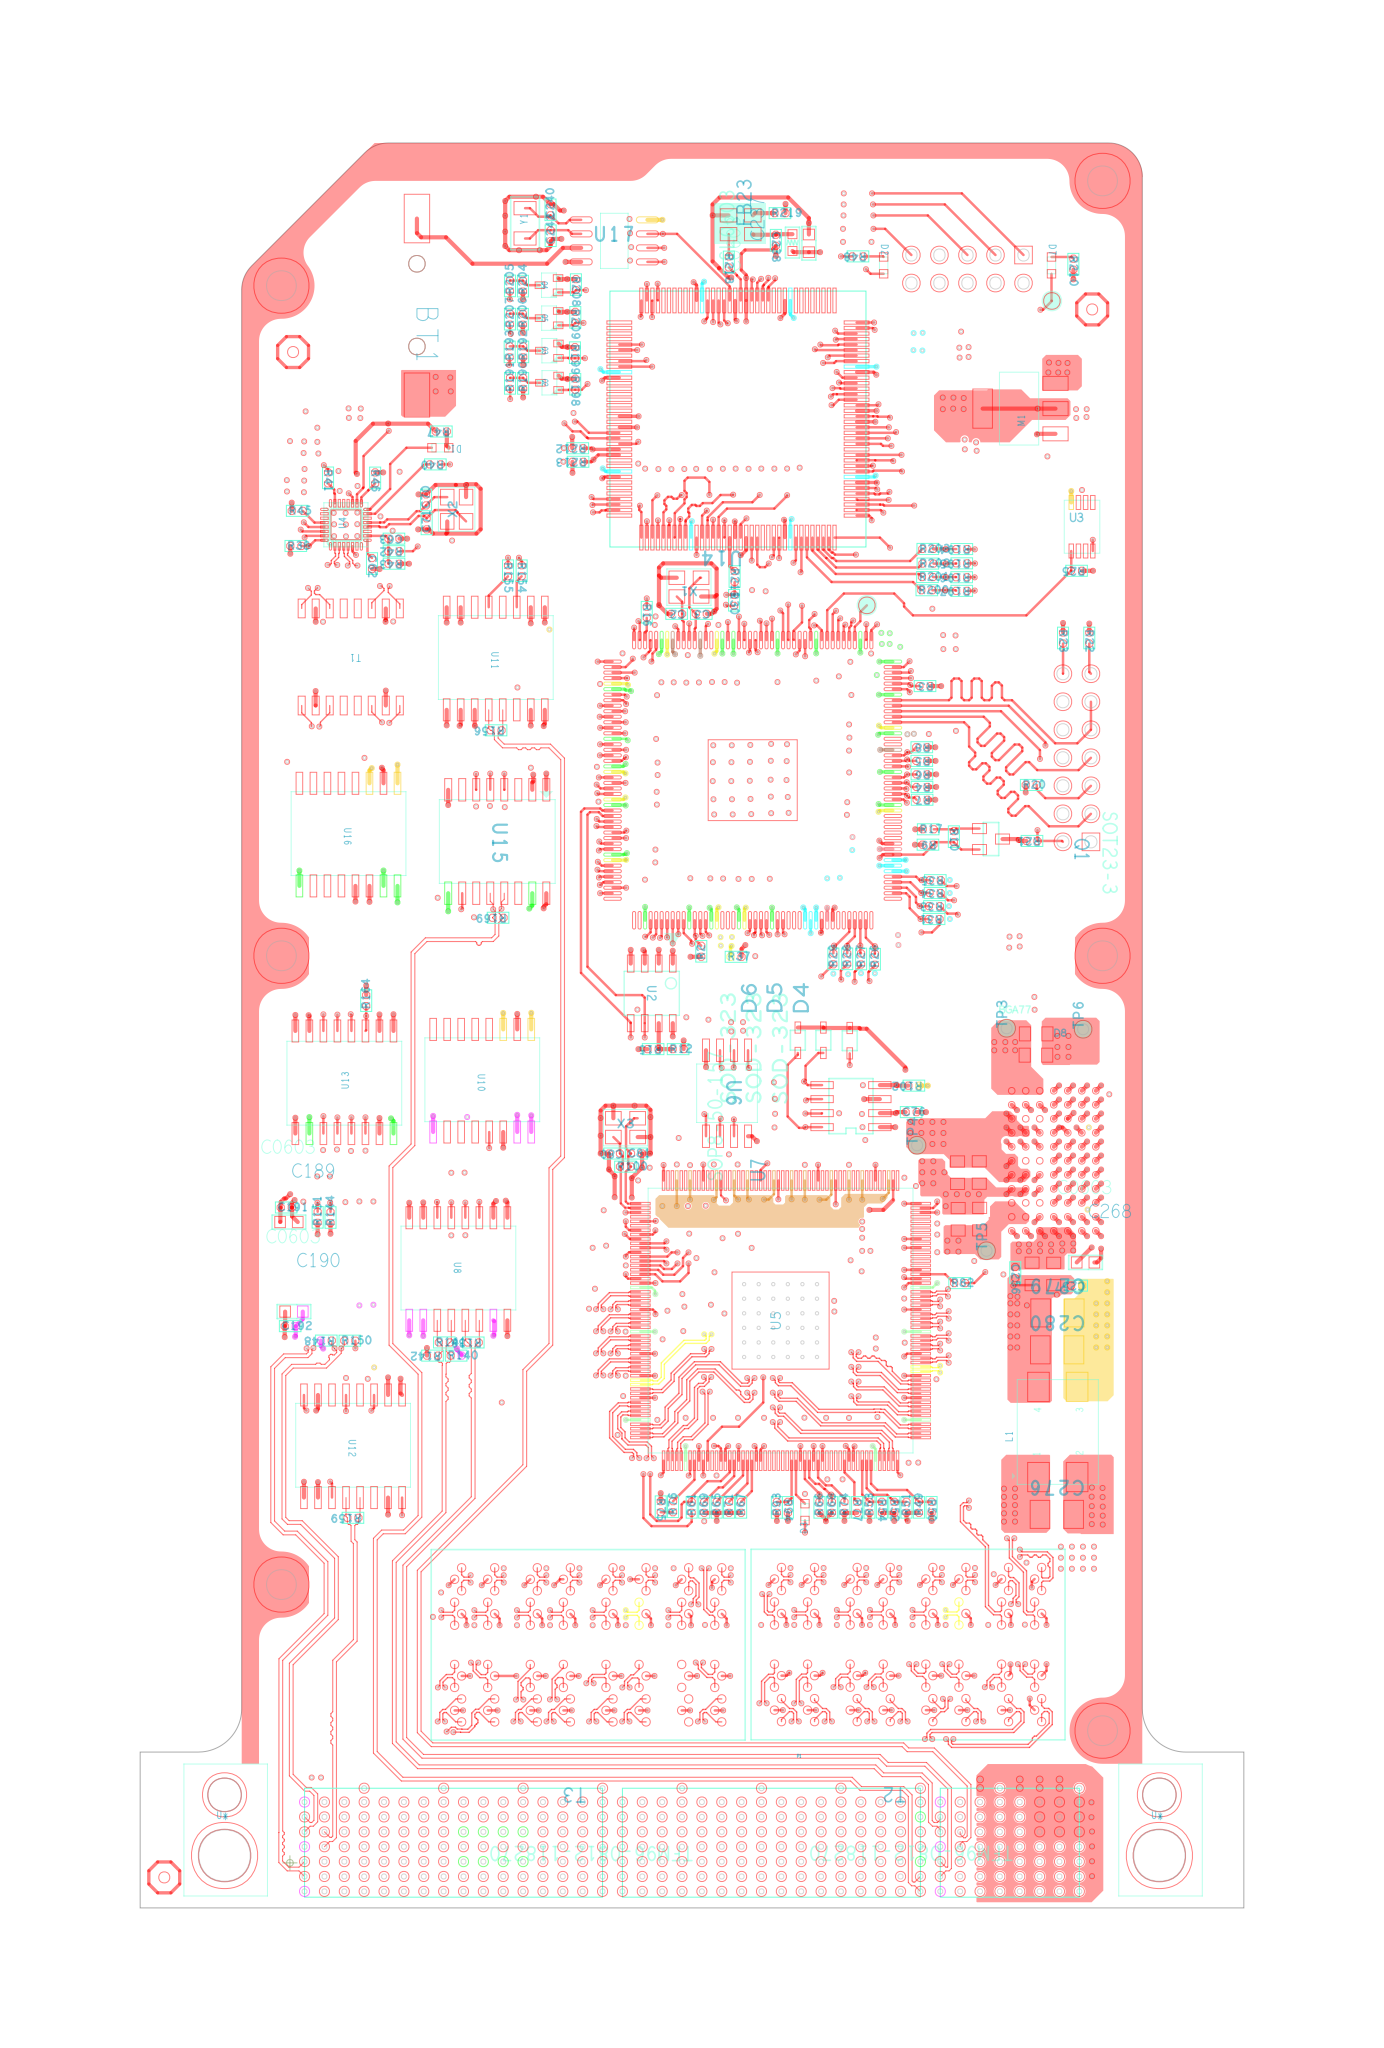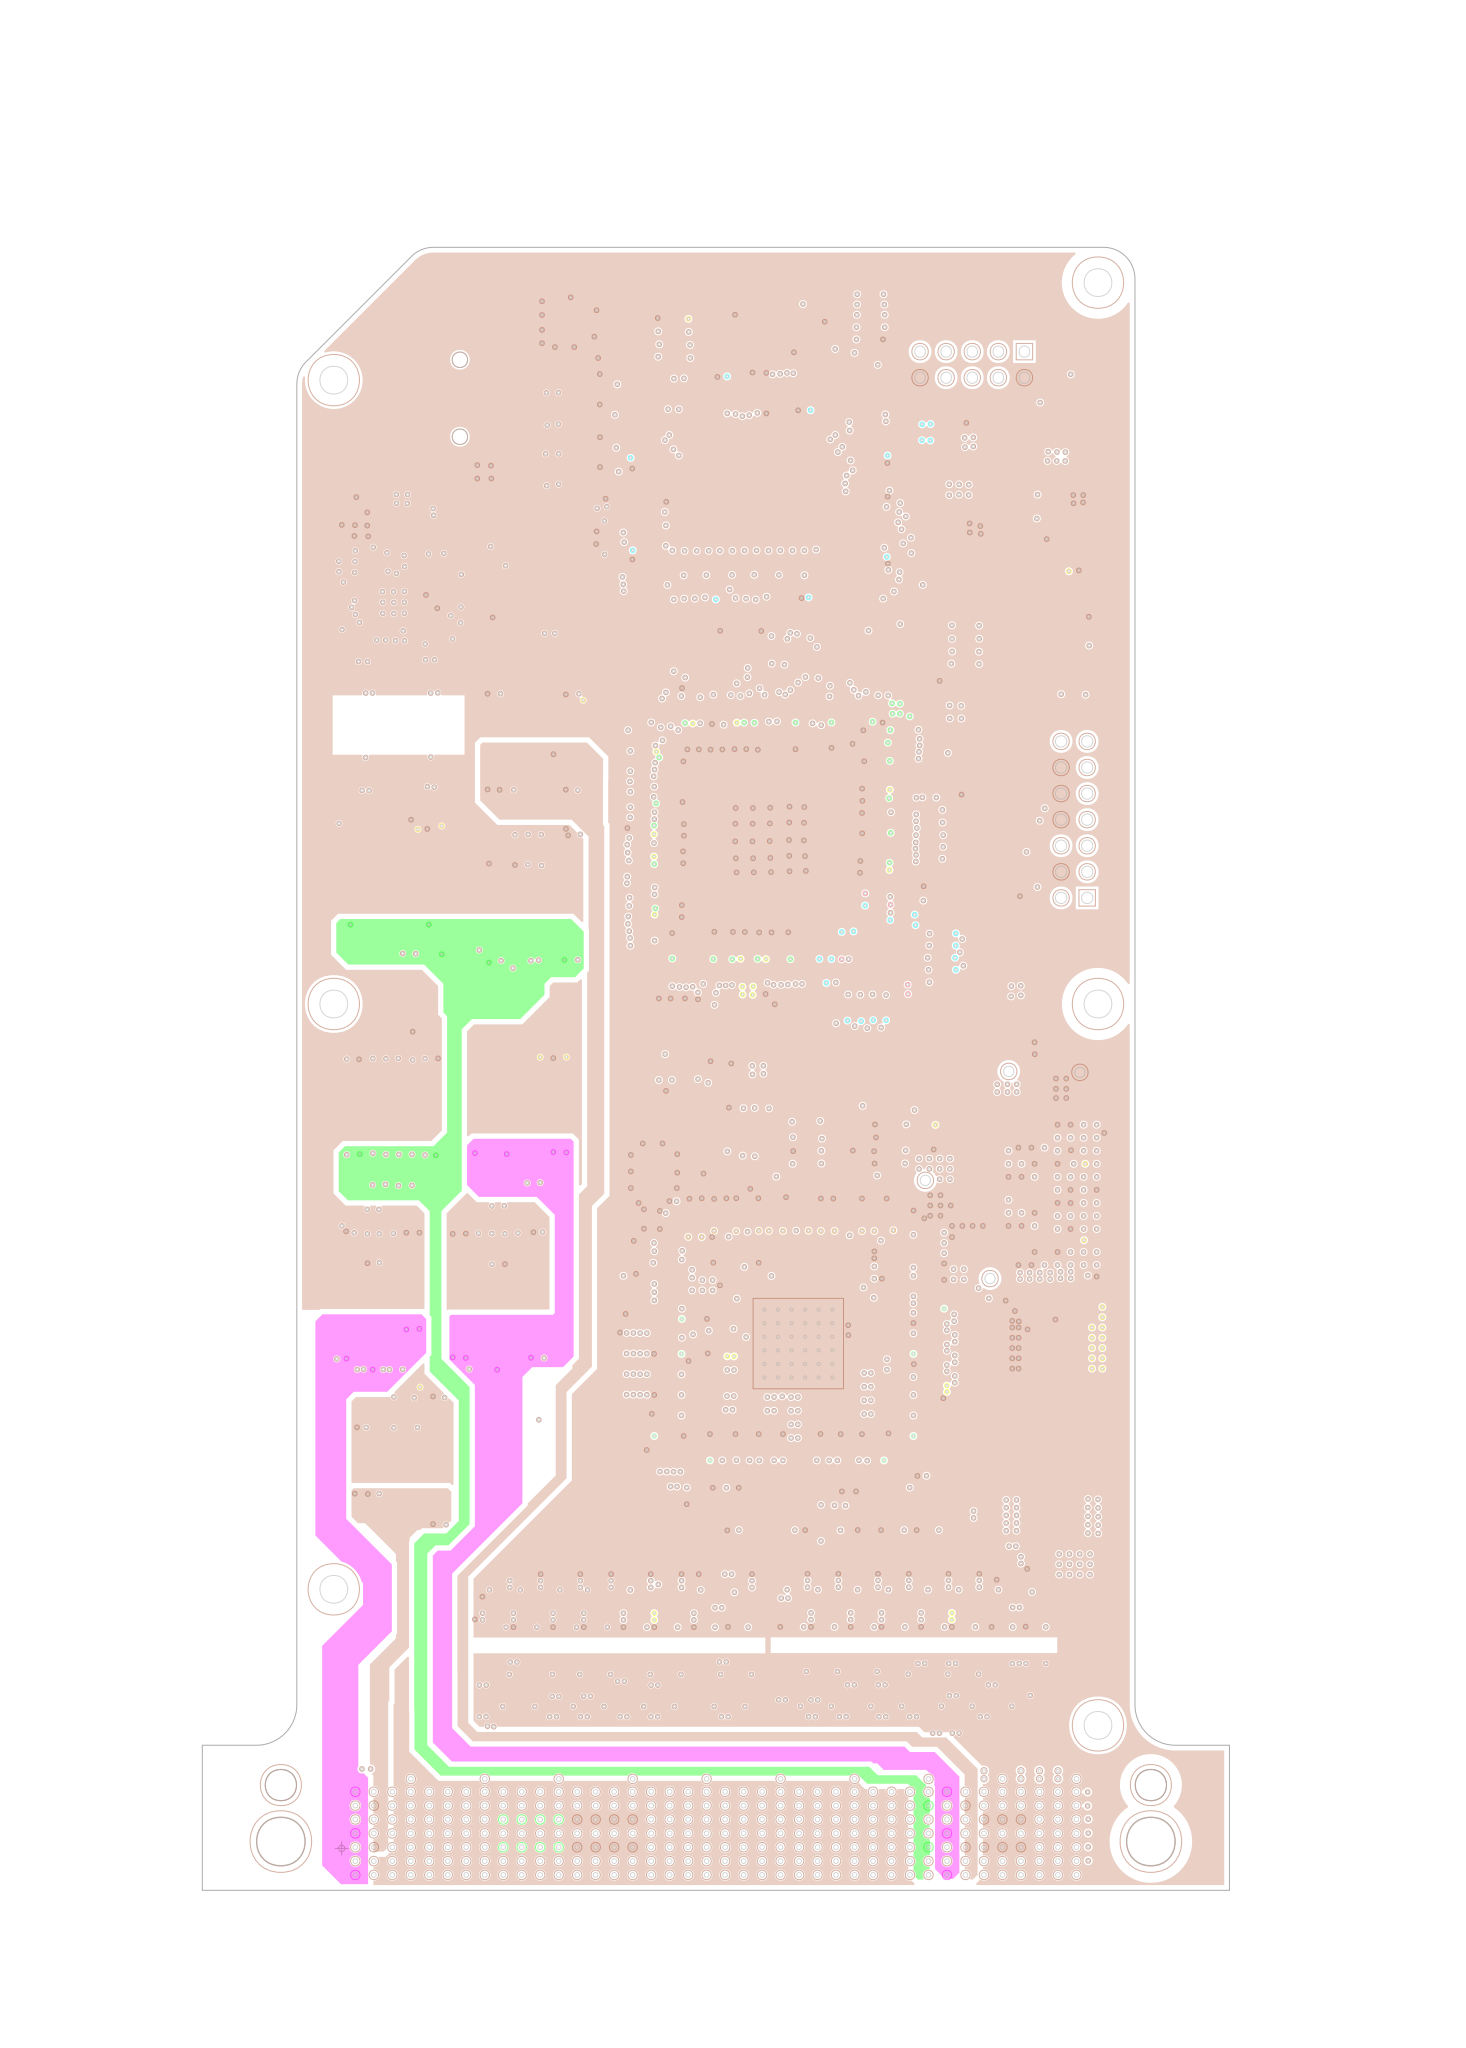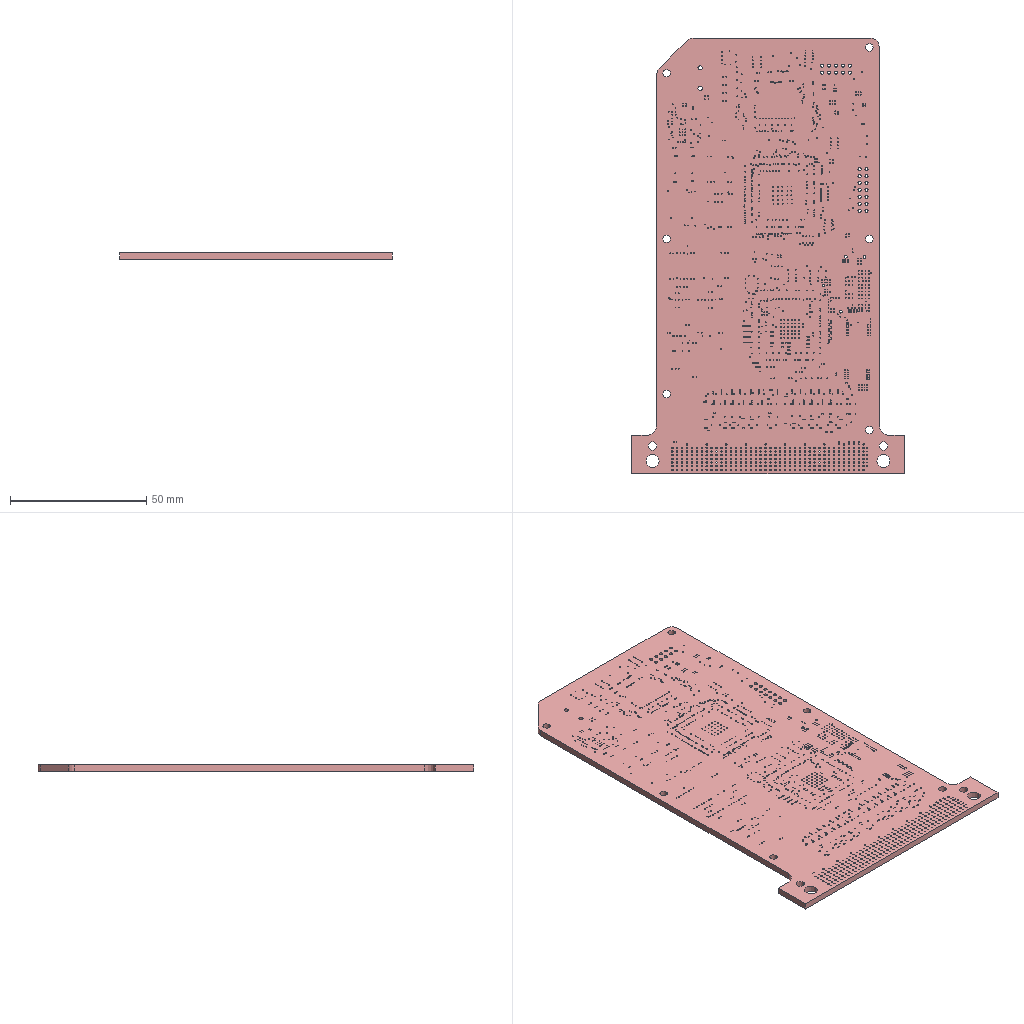Circuit board layout | Cadence Allegro | box 100 x 160 x 2.4 mm
Layer stack:
# Cadence Allegro layer stack of  (unit mm; from the constraint file cross-section; dielectric type: 0 not recorded (Allegro does not mark core vs prepreg), 3 surface material)
index,name,kind,layer,copper_thickness_mm,dielectric_type,dielectric_thickness_mm,dielectric_material,dielectric_constant
0,Top Surface,other,,,,,,
1,TOP,copper,TOP,0.0419,,,,
2,Dielectric1,dielectric,,,0,0.1148,FR-4,4.5
3,GND02,copper,GND02,0.0305,,,,
4,Dielectric2,dielectric,,,0,0.2032,FR-4,4.5
5,GND03,copper,GND03,0.0099,,,,
6,Dielectric3,dielectric,,,0,0.13,FR-4,4.5
7,ART04,copper,ART04,0.0099,,,,
8,Dielectric4,dielectric,,,0,0.22,FR-4,4.5
9,GND05,copper,GND05,0.03,,,,
10,Dielectric5,dielectric,,,0,0.2032,FR-4,4.5
11,GND06,copper,GND06,0.0305,,,,
12,Dielectric6,dielectric,,,0,0.13,FR-4,4.5
13,ART07,copper,ART07,0.03,,,,
14,Dielectric7,dielectric,,,0,0.2032,FR-4,4.5
15,POWER08,copper,POWER08,0.0305,,,,
16,Dielectric8,dielectric,,,0,0.13,FR-4,4.5
17,GND09,copper,GND09,0.03,,,,
18,Dielectric9,dielectric,,,0,0.2032,FR-4,4.5
19,ART10,copper,ART10,0.0305,,,,
20,Dielectric10,dielectric,,,0,0.1001,FR-4,4.5
21,GND11,copper,GND11,0.03,,,,
22,Dielectric11,dielectric,,,0,0.22,FR-4,4.5
23,ART12,copper,ART12,0.0099,,,,
24,Dielectric12,dielectric,,,0,0.13,FR-4,4.5
25,GND13,copper,GND13,0.0099,,,,
26,Dielectric13,dielectric,,,0,0.1148,FR-4,4.5
27,BOTTOM,copper,BOTTOM,0.0419,,,,
28,Bottom Surface,other,,,,,,
# drill layer pairs: low layer,high layer
drill_pair,TOP,BOTTOM
Part placement, first 499 of 599 lines:
REFDES,COMP_VALUE,SYM_NAME,SYM_X,SYM_Y,SYM_ROTATE,SYM_MIRROR
BT1,CR1220,CR1220,453.1,5553.8,270.000,NO
C1,0.1uF/16V,SC0402,1366.6,2998.3,270.000,YES
C2,20pF/16V,SC0402,1379.3,4458.0,180.000,NO
C3,20pF/16V,SC0402,1467.4,4458.0,180.000,NO
C4,10uF/16V,SC0603,1868.5,3360.8,0.000,YES
C5,10uF/16V,SC0603,2146.8,3564.5,90.000,YES
C6,0.1uF/16V,SC0402,1961.8,3461.0,270.000,YES
C7,0.1uF/16V,SC0402,2805.8,4856.2,180.000,YES
C8,1nF/16V,SC0402,1938.5,3226.7,270.000,YES
C9,1nF/16V,SC0402,1987.9,3226.8,270.000,YES
C10,1uF/16V,SC0402,1387.9,4364.1,270.000,YES
C11,1nF/16V,SC0402,2301.8,3507.4,0.000,YES
C12,1nF/16V,SC0402,2037.2,3226.2,270.000,YES
C13,1nF/16V,SC0402,2297.4,3368.6,0.000,YES
C14,1nF/16V,SC0402,2301.4,3461.3,0.000,YES
C15,1nF/16V,SC0402,2086.6,3225.2,270.000,YES
C16,1nF/16V,SC0402,2298.7,3414.5,0.000,YES
C17,0.1uF/16V,SC0402,1266.6,3460.3,270.000,YES
C18,0.1uF/16V,SC0402,2053.6,4351.3,180.000,YES
C19,0.1uF/16V,SC0402,2046.6,4282.7,0.000,YES
C20,0.1uF/16V,SC0402,2052.8,4168.3,0.000,YES
C21,0.1uF/16V,SC0402,1595.2,4260.6,90.000,YES
C22,0.1uF/16V,SC0402,1877.6,4270.2,90.000,YES
C23,0.1uF/16V,SC0402,1600.1,3465.3,270.000,YES
C24,0.1uF/16V,SC0402,1254.9,3777.1,180.000,YES
C25,0.1uF/16V,SC0402,1263.2,4167.6,180.000,YES
C26,0.1uF/16V,SC0402,1255.1,3927.1,180.000,YES
C27,0.1uF/16V,SC0402,1256.0,3616.6,180.000,YES
C28,0.1uF/16V,SC0402,1550.7,4261.0,90.000,YES
C29,0.1uF/16V,SC0402,1428.3,3466.2,270.000,YES
C30,0.1uF/16V,SC0402,2048.5,3785.7,0.000,YES
C31,10uF/16V,SC0603,2291.7,4408.3,270.000,YES
C32,10uF/16V,SC0603,2028.7,4234.8,0.000,YES
C33,0.1uF/16V,SC0402,2046.9,4016.2,0.000,YES
C34,0.1uF/16V,SC0402,1739.3,4268.8,90.000,YES
C35,0.1uF/16V,SC0402,1253.7,4011.5,180.000,YES
C36,0.1uF/16V,SC0402,1325.0,4260.6,90.000,YES
C37,0.1uF/16V,SC0402,1711.8,3465.8,270.000,YES
C38,0.1uF/16V,SC0402,1499.7,3466.1,270.000,YES
C39,0.1uF/16V,SC0402,2050.0,3891.8,0.000,YES
C40,1uF/16V,SC0402,2356.1,4072.6,180.000,YES
C41,1uF/16V,SC0402,1459.0,4260.8,90.000,YES
C42,0.1uF/16V,SC0402,2047.4,3969.9,0.000,YES
C43,0.1uF/16V,SC0402,1414.0,4260.8,90.000,YES
C44,10uF/16V,SC0603,1524.4,3051.8,0.000,YES
C45,10uF/16V,SC0603,1593.2,3236.2,180.000,YES
C46,0.1uF/16V,SC0402,1262.8,4213.4,180.000,YES
C47,0.1uF/16V,SC0402,2048.5,3740.6,0.000,YES
C48,0.1uF/16V,SC0402,2047.4,4061.3,0.000,YES
C49,0.1uF/16V,SC0402,1505.7,4261.2,90.000,YES
C50,0.1uF/16V,SC0402,1254.9,3822.7,180.000,YES
C51,0.1uF/16V,SC0402,1647.3,3465.3,270.000,YES
C52,0.1uF/16V,SC0402,1255.5,3882.7,180.000,YES
C53,0.1uF/16V,SC0402,1545.3,3465.2,270.000,YES
C54,0.1uF/16V,SC0402,1369.1,4261.0,90.000,YES
C55,0.1uF/16V,SC0402,1256.4,3570.7,180.000,YES
C56,10uF/16V,SC0603,2523.4,3208.5,90.000,YES
C57,0.1uF/16V,SC0402,2576.5,3203.1,90.000,YES
C58,10uF/16V,SC0603,2304.3,3211.0,90.000,YES
C59,1uF/16V,SC0402,2055.4,3614.7,0.000,YES
C60,0.1uF/16V,SC0402,1916.7,3460.8,270.000,YES
C61,1uF/16V,SC0402,361.2,4458.8,0.000,YES
C62,1uF/16V,SC0402,292.8,4637.4,270.000,NO
C63,1uF/16V,SC0402,371.0,4726.3,180.000,NO
C64,1uF/16V,SC0402,110.4,4457.4,0.000,YES
C65,1000pF/2kV,SC1812,-7.0,4034.3,270.000,YES
C66,10uF/16V,SC0603,130.2,5180.5,0.000,YES
C67,0.1uF/16V,SC0402,151.7,5122.3,0.000,YES
C68,10uF/16V,SC0603,332.6,5002.1,180.000,YES
C69,0.1uF/16V,SC0402,319.3,4931.6,180.000,YES
C70,20pF/16V,SC0402,485.6,4864.6,90.000,NO
C71,20pF/16V,SC0402,487.7,4779.1,90.000,NO
C72,10uF/16V,SC0603,196.2,5001.9,0.000,YES
C73,0.1uF/16V,SC0402,197.2,4931.7,0.000,YES
C74,0.1uF/16V,SC0402,1615.3,2573.9,0.000,YES
C75,1uF/16V,SC0402,1614.9,2528.7,0.000,YES
C76,1uF/16V,SC0402,2216.1,2679.6,0.000,NO
C77,0.1uF/16V,SC0402,2109.1,2672.9,0.000,YES
C78,1uF/16V,SC0402,2110.7,2625.8,0.000,YES
C79,0.1uF/16V,SC0402,1888.3,2675.4,180.000,YES
C80,27pF/16V,SC0402,1157.7,2531.7,180.000,NO
C81,27pF/16V,SC0402,1236.5,2531.7,0.000,NO
C82,10uF/16V,SC0603,1506.1,1435.5,180.000,YES
C83,0.1uF/16V,SC0402,1433.2,1269.0,90.000,YES
C84,10uF/16V,SC0603,2149.9,1936.4,270.000,YES
C85,0.1uF/16V,SC0402,1333.2,1919.4,90.000,YES
C86,0.1uF/16V,SC0402,1253.8,1817.4,0.000,YES
C87,0.1uF/16V,SC0402,2166.9,1460.6,180.000,YES
C88,0.1uF/16V,SC0402,1253.8,1659.9,0.000,YES
C89,0.1uF/16V,SC0402,1458.9,1541.5,270.000,YES
C90,0.1uF/16V,SC0402,1352.6,1437.3,180.000,YES
C91,0.1uF/16V,SC0402,2226.7,1994.6,270.000,YES
C92,0.1uF/16V,SC0402,2249.2,1807.4,180.000,YES
C93,0.1uF/16V,SC0402,2119.5,1660.2,0.000,YES
C94,10uF/16V,SC0603,1261.3,1530.4,180.000,YES
C95,0.1uF/16V,SC0402,1350.8,2030.0,180.000,YES
C96,0.1uF/16V,SC0402,2226.7,1876.4,90.000,YES
C97,0.1uF/16V,SC0402,2252.8,2052.7,0.000,YES
C98,0.1uF/16V,SC0402,1259.9,1581.2,180.000,YES
C99,0.1uF/16V,SC0402,1411.6,1541.5,270.000,YES
C100,0.1uF/16V,SC0402,2191.3,1526.1,90.000,YES
C101,0.1uF/16V,SC0402,2095.5,1541.5,270.000,YES
C102,0.1uF/16V,SC0402,1253.8,1896.1,0.000,YES
C103,10uF/16V,SC0603,1388.4,2306.0,180.000,YES
C104,0.1uF/16V,SC0402,2127.5,2184.3,0.000,YES
C105,0.1uF/16V,SC0402,1994.3,1541.5,270.000,YES
C106,0.1uF/16V,SC0402,2124.3,2083.0,0.000,YES
C107,0.1uF/16V,SC0402,1553.4,1541.5,270.000,YES
C108,0.1uF/16V,SC0402,1868.3,1541.5,270.000,YES
C109,0.1uF/16V,SC0402,1350.8,2079.4,180.000,YES
C110,0.1uF/16V,SC0402,1823.5,1541.5,270.000,YES
C111,0.1uF/16V,SC0402,2129.5,2339.8,0.000,YES
C112,0.1uF/16V,SC0402,1393.8,2218.3,180.000,YES
C113,0.1uF/16V,SC0402,1644.6,1541.5,270.000,YES
C114,10uF/16V,SC0603,2045.5,1573.4,270.000,YES
C115,10uF/16V,SC0603,2113.4,2289.0,0.000,YES
C116,0.1uF/16V,SC0402,2252.8,2226.7,180.000,YES
C117,0.1uF/16V,SC0402,2252.4,2156.0,180.000,YES
C118,0.1uF/16V,SC0402,1166.1,2199.4,270.000,YES
C119,0.1uF/16V,SC0402,1912.5,1541.5,270.000,YES
C120,0.1uF/16V,SC0402,1691.3,1541.5,270.000,YES
C121,0.1uF/16V,SC0402,1166.1,2309.5,270.000,YES
C122,0.1uF/16V,SC0402,1243.5,2328.0,180.000,YES
C123,0.1uF/16V,SC0402,2252.4,2116.6,180.000,YES
C124,0.1uF/16V,SC0402,2252.8,2384.3,0.000,YES
C125,0.1uF/16V,SC0402,1166.1,2120.6,270.000,YES
C126,0.1uF/16V,SC0402,1509.5,1541.5,270.000,YES
C127,0.1uF/16V,SC0402,1779.0,1541.5,270.000,YES
C128,0.1uF/16V,SC0402,1598.5,1541.5,270.000,YES
C129,10uF/16V,SC0603,1380.1,2415.8,270.000,YES
C130,10uF/16V,SC0603,1328.5,2417.2,270.000,YES
C131,0.1uF/16V,SC0402,1472.8,2415.8,270.000,YES
C132,0.1uF/16V,SC0402,1994.3,2415.8,270.000,YES
C133,0.1uF/16V,SC0402,1598.8,2415.8,270.000,YES
C134,0.1uF/16V,SC0402,2131.7,2415.3,270.000,YES
C135,0.1uF/16V,SC0402,1512.2,2415.8,270.000,YES
C136,0.1uF/16V,SC0402,1427.4,2415.8,270.000,YES
C137,0.1uF/16V,SC0402,2041.5,2415.8,270.000,YES
C138,0.1uF/16V,SC0402,1644.1,2415.8,270.000,YES
C139,0.1uF/16V,SC0402,1703.1,2415.6,270.000,YES
C140,0.1uF/16V,SC0402,1836.8,2415.8,270.000,YES
C141,0.1uF/16V,SC0402,1789.6,2415.8,270.000,YES
C142,0.1uF/16V,SC0402,1906.1,2415.7,270.000,YES
C143,10uF/16V,SC0603,1967.2,2258.4,180.000,YES
C144,0.1uF/16V,SC0402,2086.9,2415.5,270.000,YES
C145,0.1uF/16V,SC0402,1950.3,2415.3,270.000,YES
C146,0.1uF/16V,SC0402,1555.5,2416.3,270.000,YES
C147,0.1uF/16V,SC0402,1747.1,2415.7,270.000,YES
C148,10uF/16V,SC0603,1979.2,1940.5,270.000,YES
C149,0.1uF/16V,SC0402,1253.8,1738.7,0.000,YES
C150,0.1uF/16V,SC0402,2249.2,1739.2,180.000,YES
C151,0.1uF/16V,SC0402,2677.9,1032.9,90.000,YES
C152,0.1uF/16V,SC0402,2543.7,1032.5,90.000,YES
C153,0.1uF/16V,SC0402,1402.8,889.2,180.000,YES
C154,0.1uF/16V,SC0402,1535.5,1031.9,90.000,YES
C155,0.1uF/16V,SC0402,2661.8,890.2,180.000,YES
C156,0.1uF/16V,SC0402,1520.8,889.2,180.000,YES
C157,0.1uF/16V,SC0402,1397.5,1031.9,90.000,YES
C158,0.1uF/16V,SC0402,2543.8,890.2,180.000,YES
C159,0.1uF/16V,SC0402,2386.5,1032.9,90.000,YES
C160,0.1uF/16V,SC0402,1245.5,1031.9,90.000,YES
C161,0.1uF/16V,SC0402,2391.8,890.2,180.000,YES
C162,0.1uF/16V,SC0402,1250.8,889.2,180.000,YES
C163,0.1uF/16V,SC0402,2268.5,1032.9,90.000,YES
C164,0.1uF/16V,SC0402,1127.5,1031.9,90.000,YES
C165,0.1uF/16V,SC0402,2273.8,890.2,180.000,YES
C166,0.1uF/16V,SC0402,1132.8,889.2,180.000,YES
C167,0.1uF/16V,SC0402,2116.5,1032.9,90.000,YES
C168,0.1uF/16V,SC0402,975.5,1031.9,90.000,YES
C169,0.1uF/16V,SC0402,2121.8,890.2,180.000,YES
C170,0.1uF/16V,SC0402,980.8,889.2,180.000,YES
C171,0.1uF/16V,SC0402,1998.5,1032.9,90.000,YES
C172,0.1uF/16V,SC0402,857.5,1031.9,90.000,YES
C173,0.1uF/16V,SC0402,2003.8,890.2,180.000,YES
C174,0.1uF/16V,SC0402,862.8,889.2,180.000,YES
C175,0.1uF/16V,SC0402,1846.5,1032.9,90.000,YES
C176,0.1uF/16V,SC0402,705.5,1031.9,90.000,YES
C177,0.1uF/16V,SC0402,1851.8,890.2,180.000,YES
C178,0.1uF/16V,SC0402,710.8,889.2,180.000,YES
C179,0.1uF/16V,SC0402,1728.5,1032.9,90.000,YES
C180,0.1uF/16V,SC0402,587.5,1031.9,90.000,YES
C181,0.1uF/16V,SC0402,1733.8,890.2,180.000,YES
C182,0.1uF/16V,SC0402,592.8,889.2,180.000,YES
C183,1000pF/2kV,SC1812,2869.8,709.9,90.000,YES
C184,1000pF/2kV,SC1812,365.8,544.2,0.000,YES
C185,10uF/16V,SC0603,751.3,2279.4,0.000,YES
C186,10uF/16V,SC0603,749.7,1958.7,0.000,YES
C187,0.1uF/16V,SC0402,755.9,2329.1,0.000,YES
C188,0.1uF/16V,SC0402,748.7,1908.8,0.000,YES
C189,10uF/16V,SC0603,-3.6,2287.2,0.000,NO
C190,10uF/16V,SC0603,14.4,1967.6,0.000,NO
C191,0.1uF/16V,SC0402,-13.1,2339.2,0.000,NO
C192,0.1uF/16V,SC0402,1.1,1915.6,0.000,NO
C193,10uF/16V,SC0603,796.8,2989.7,0.000,YES
C194,0.1uF/16V,SC0402,822.2,2582.9,180.000,YES
C195,10uF/16V,SC0603,808.5,2634.2,180.000,YES
C196,0.1uF/16V,SC0402,835.1,3061.4,180.000,YES
C197,10uF/16V,SC0603,883.7,4507.7,0.000,YES
C198,1uF/16V,SC0402,886.2,4455.6,0.000,YES
C199,0.1uF/16V,SC0402,882.4,4095.7,0.000,YES
C200,10uF/16V,SC0603,876.2,4204.3,0.000,YES
C201,1uF/16V,SC0402,635.8,4086.6,0.000,YES
C202,1uF/16V,SC0402,585.0,4460.0,180.000,YES
C203,10uF/16V,SC0603,372.7,1637.5,0.000,YES
C204,1uF/16V,SC0402,375.0,1689.7,0.000,YES
C205,10uF/16V,SC0603,379.4,1334.7,0.000,YES
C206,1uF/16V,SC0402,124.4,1327.7,0.000,YES
C207,0.1uF/16V,SC0402,379.3,1282.8,0.000,YES
C208,1uF/16V,SC0402,74.7,1652.4,180.000,YES
C209,0.1uF/16V,SC0402,46.9,2993.3,0.000,YES
C210,0.1uF/16V,SC0402,42.3,2629.0,180.000,YES
C211,1uF/16V,SC0402,345.4,2991.3,0.000,YES
C212,1uF/16V,SC0402,345.0,2627.6,0.000,YES
C213,0.1uF/16V,SC0402,889.7,3848.7,0.000,YES
C214,0.1uF/16V,SC0402,894.1,3456.7,0.000,YES
C215,10uF/16V,SC0603,309.9,3820.2,0.000,YES
C216,0.1uF/16V,SC0402,340.9,3465.6,180.000,YES
C217,10uF/16V,SC0603,333.2,3385.9,180.000,YES
C218,0.1uF/16V,SC0402,308.2,3873.8,0.000,YES
C219,0.1uF/16V,SC0402,1146.3,5309.8,90.000,YES
C220,0.1uF/16V,SC0402,1456.4,5605.8,0.000,YES
C221,10uF/16V,SC0603,2326.4,5465.3,180.000,YES
C222,0.1uF/16V,SC0402,1776.4,5545.2,0.000,YES
C223,0.1uF/16V,SC0402,1438.4,4730.3,90.000,YES
C224,0.1uF/16V,SC0402,2048.5,5330.3,90.000,YES
C225,0.1uF/16V,SC0402,1150.1,4958.5,90.000,YES
C226,0.1uF/16V,SC0402,1774.8,4759.4,0.000,YES
C227,0.1uF/16V,SC0402,2050.8,4935.7,90.000,YES
C228,0.1uF/16V,SC0402,1211.0,5140.7,270.000,YES
C229,0.1uF/16V,SC0402,2052.7,5160.8,270.000,YES
C230,10uF/16V,SC0603,2000.6,5159.1,270.000,YES
C231,0.1uF/16V,SC0402,1589.3,4735.5,90.000,YES
C232,0.1uF/16V,SC0402,1608.2,5537.4,180.000,YES
C233,10uF/16V,SC0603,2758.6,5231.8,90.000,YES
C234,0.1uF/16V,SC0402,2808.3,5238.6,90.000,YES
C235,0.1uF/16V,SC0402,2403.3,5135.8,90.000,YES
C236,10uF/16V,SC0603,2459.3,5134.4,90.000,YES
C237,10uF/16V,SC0603,1851.3,5780.3,90.000,NO
C238,0.1uF/16V,SC0402,1733.4,5791.3,270.000,NO
C239,1uF/16V,SC0402,2025.9,5785.5,180.000,YES
C240,10pF/16V,SC0402,929.5,5900.1,90.000,NO
C241,0.1uF/16V,SC0402,1271.1,5867.3,0.000,YES
C242,10pF/16V,SC0402,930.1,5807.6,90.000,NO
C243,47uF/10V,SC0805,2662.1,2958.8,0.000,NO
C244,47uF/10V,SC0805,2661.2,2882.8,0.000,NO
C245,0.1uF/16V,SC0402,2639.0,2955.4,180.000,YES
C246,1nF/16V,SC0402,2639.6,2895.8,180.000,YES
C247,47uF/10V,SC0805,2459.1,2464.0,270.000,NO
C248,47uF/10V,SC0805,2381.6,2463.4,270.000,NO
C249,0.1uF/16V,SC0402,2389.2,2486.8,90.000,YES
C250,1nF/16V,SC0402,2442.6,2486.5,90.000,YES
C251,22uF/16V,SC0805,2647.4,2102.1,270.000,NO
C252,22uF/16V,SC0805,2698.0,2094.0,90.000,YES
C253,22uF/16V,SC0805,2620.8,2094.4,90.000,YES
C254,22uF/16V,SC0805,2724.5,2101.7,270.000,NO
C255,22uF/16V,SC0805,2831.0,2058.1,0.000,YES
C256,1uF/16V,SC0402,2587.5,2106.9,270.000,NO
C257,0.1uF/16V,SC0402,2806.4,2060.2,180.000,NO
C258,47uF/10V,SC0805,2383.9,2297.0,90.000,NO
C259,47uF/10V,SC0805,2460.3,2297.6,90.000,NO
C260,0.1uF/16V,SC0402,2443.8,2275.7,270.000,YES
C261,1nF/16V,SC0402,2389.0,2275.3,270.000,YES
C262,4.7uF/16V,SC0603,2702.3,2467.5,90.000,YES
C263,0.1uF/16V,SC0402,2716.8,2728.6,90.000,YES
C264,0.1uF/16V,SC0402,2819.6,2573.2,90.000,YES
C265,0.1uF/16V,SC0402,2794.3,2401.5,180.000,YES
C266,0.1uF/16V,SC0402,2793.9,2262.3,180.000,YES
C267,10pF/16V,SC0402,2846.0,2700.0,0.000,YES
C268,4.7uF/16V,SC0603,2838.1,2143.0,0.000,NO
C269,10pF/16V,SC0402,2870.4,2473.8,270.000,YES
C270,10nF/16V,SC0402,2793.7,2749.9,180.000,YES
C271,10pF/16V,SC0402,2925.4,2226.5,90.000,YES
C272,10nF/16V,SC0402,2794.7,2449.7,180.000,YES
C273,10nF/16V,SC0402,2792.8,2315.3,180.000,YES
C274,4.7uF/16V,SC0603,2702.3,2587.5,90.000,YES
C275,100uF/16V,C1210,2727.1,1279.4,0.000,YES
C276,100uF/16V,C1210,2735.7,1243.8,180.000,NO
C277,4.7nF/1kV,C1812,2808.1,1533.2,270.000,YES
C278,4.7nF/1kV,C1812,2805.7,1840.7,90.000,YES
C279,100uF/16V,C1210,2737.9,1962.9,180.000,NO
C280,100uF/16V,C1210,2736.9,1831.1,180.000,NO
C281,4.7nF/1kV,C1812,2664.2,1534.4,90.000,YES
C282,4.7nF/1kV,C1812,2666.6,1838.4,270.000,YES
D1,G-LED,D0603,536.4,5050.7,180.000,NO
D2,G-LED,D0603,2118.0,5701.6,270.000,NO
D3,G-LED,D0603,1837.3,1252.0,90.000,NO
D4,B5817W,SOD-323,1997.0,2934.5,90.000,NO
D5,B5817W,SOD-323,1902.9,2936.0,90.000,NO
D6,B5817W,SOD-323,1811.8,2936.0,90.000,NO
D7,G-LED,D0603,2716.7,5701.6,270.000,NO
D8,LTM4644IY#PBF,BGA77-1R27-15X9,2724.8,2505.7,0.000,NO
FB1,PZ1608D600-2R0TF,SL0603,1367.6,4448.7,180.000,YES
FB2,PZ1608D600-2R0TF,SL0603,2202.2,4375.1,0.000,YES
FB3,PZ1608D600-2R0TF,SL0603,2248.7,4072.6,0.000,YES
FB4,PZ1608D600-2R0TF,SL0603,1561.4,3145.1,270.000,YES
FB5,PZ1608D600-2R0TF,SL0603,2417.1,3242.7,0.000,YES
FB6,PZ1608D600-2R0TF,SL0603,2413.1,3139.1,0.000,YES
FB7,PZ1608D600-2R0TF,SL0603,2411.6,3082.5,0.000,YES
FB8,PZ1608D600-2R0TF,SL0603,296.7,5091.2,90.000,YES
FB9,PZ1608D600-2R0TF,SL0603,9.7,5010.0,90.000,YES
FB10,PZ1608D600-2R0TF,SL0603,229.3,5091.2,90.000,YES
FB11,PZ1608U121-1R0TF,SL0603,2094.7,1940.8,90.000,YES
FB12,PZ1608U121-1R0TF,SL0603,2241.4,1515.8,270.000,YES
FB13,PZ1608D300-3R0TF,SL0603,2111.1,2133.2,180.000,YES
FB14,PZ1608U121-1R0TF,SL0603,2115.5,2233.7,180.000,YES
FB15,PZ1608U121-1R0TF,SL0603,1272.5,2418.7,90.000,YES
FB16,PZ1608U121-1R0TF,SL0603,1965.7,2201.5,0.000,YES
FB17,PZ1608U121-1R0TF,SL0603,2039.4,1940.6,90.000,YES
FB18,PZ1608U121-1R0TF,SL0603,974.0,4476.7,270.000,YES
FB19,PZ1608U121-1R0TF,SL0603,872.0,4148.5,180.000,YES
FB20,PZ1608U121-1R0TF,SL0603,370.0,1768.3,180.000,YES
FB21,PZ1608U121-1R0TF,SL0603,378.5,1390.5,180.000,YES
FB22,PZ1608D600-2R0TF,SL0603,2321.9,5402.6,0.000,YES
FB23,PZ1608D600-2R0TF,SL0603,1792.7,5783.0,90.000,NO
FB24,PZ3216U300-6R0TF,FB1206,2901.8,2140.7,0.000,YES
H1,screw-d5-d2p8,SCREW-D5-D2P8,-30.3,993.3,0.000,NO
H2,screw-d5-d2p8,SCREW-D5-D2P8,2898.8,471.7,0.000,NO
H3,screw-d5-d2p8,SCREW-D5-D2P8,2898.8,3237.4,0.000,NO
H4,screw-d5-d2p8,SCREW-D5-D2P8,-30.3,3237.4,0.000,NO
H5,screw-d5-d2p8,SCREW-D5-D2P8,2898.8,6003.2,0.000,NO
H6,screw-d5-d2p8,SCREW-D5-D2P8,-30.3,5629.2,0.000,NO
J1,DSP_JTAG,HC-PZ254-2X7PZ,2807.4,3944.2,90.000,NO
J2,CPLD_JTAG,HC-PZ254-2X5PWA,2416.9,5688.6,180.000,NO
L1,LCM9070-501,LCM9070,2739.2,1537.9,90.000,NO
M1,BL1117-CX,SOT-223-4,2731.0,5100.4,90.000,NO
P1,JVPX-21T8aAC8-B,JVPX-21T8AAC8-B,2816.1,-101.7,0.000,NO
Q1,XCA431BHA,SOT23-3,2500.9,3654.1,270.000,NO
Q2,WNM6002-3/TR,SOT_323,925.7,5282.6,270.000,NO
Q3,WNM6002-3/TR,SOT_323,925.4,5397.2,270.000,NO
Q4,WNM6002-3/TR,SOT_323,924.0,5630.9,270.000,NO
Q5,WNM6002-3/TR,SOT_323,924.5,5513.3,270.000,NO
R1,4.7K 1%,SR0402,1152.7,4166.4,180.000,YES
R2,2.2K 1%,SR0402,1467.4,3253.7,90.000,NO
R3,4.7K 1%,SR0402,2265.4,4200.1,180.000,NO
R4,4.7K 1%,SR0402,2254.7,3840.1,180.000,NO
R5,4.7K 1%,SR0402,2253.9,3933.1,180.000,NO
R6,4.7K 1%,SR0402,2254.3,3885.0,180.000,NO
R7,4.7K 1%,SR0402,2255.1,3794.4,180.000,NO
R8,4.7K 1%,SR0402,2253.9,3981.8,180.000,NO
R9,100R 1%,SR0402,2275.9,3634.0,180.000,NO
R10,1K 1%,SR0402,2368.4,3662.6,270.000,NO
R11,2.2K 1%,SR0402,1218.0,3003.5,90.000,YES
R12,4.7K 1%,SR0402,1384.9,2904.3,0.000,NO
R13,2.2K 1%,SR0402,1264.7,3002.9,90.000,YES
R14,0R 1%,SR0402,1148.3,4287.2,0.000,YES
R15,4.7K 1%,SR0402,1295.5,2904.3,180.000,NO
R16,0R 1%,SR0402,1272.9,4463.6,270.000,NO
R17,10K 1%,SR0402,2277.0,3689.0,0.000,NO
R18,4.7K 1%,SR0402,1137.3,3807.3,270.000,YES
R19,1K 1%,SR0402,1137.1,3892.2,270.000,YES
R20,10R 1%,SR0402,2644.4,3847.3,0.000,NO
R21,2.2K 1%,SR0402,2647.0,3647.4,180.000,NO
R22,10K 1%,SR0402,2851.5,4371.7,270.000,NO
R23,10K 1%,SR0402,2757.9,4371.7,270.000,NO
R24,0R 1%,SR0402,2056.1,3661.2,0.000,YES
R25,4.7K 1%,SR0402,2806.0,4611.6,180.000,NO
R26,100R 1%,SR0402,2086.7,3225.3,90.000,NO
R27,100R 1%,SR0402,2037.5,3226.2,90.000,NO
R28,100R 1%,SR0402,1987.9,3226.7,90.000,NO
R29,100R 1%,SR0402,1938.6,3226.7,90.000,NO
R30,0R 1%,SR0402,1584.5,4506.2,270.000,NO
R31,100R 1%,SR0402,2297.7,3368.6,180.000,NO
R32,0R 1%,SR0402,1494.8,4384.3,180.000,YES
R33,100R 1%,SR0402,2299.1,3414.6,180.000,NO
R34,100R 1%,SR0402,2301.6,3461.5,180.000,NO
R35,100R 1%,SR0402,2302.1,3507.4,180.000,NO
R36,10K 1%,SR0402,1321.3,4383.2,180.000,YES
R37,82R 1%,SR0402,1591.4,3233.9,0.000,NO
R38,4.7K 1%,SR0402,21.1,4700.2,0.000,NO
R39,75R 1%,SR0402,341.7,4130.5,90.000,YES
R40,0R 1%,SR0402,518.7,4991.3,180.000,NO
R41,0R 1%,SR0402,136.0,4943.3,270.000,NO
R42,0R 1%,SR0402,371.0,4681.5,180.000,NO
R43,10K 1%,SR0402,371.3,4636.8,180.000,NO
R44,75R 1%,SR0402,91.7,4131.2,90.000,YES
R45,1K 1%,SR0402,26.1,4825.6,0.000,NO
R46,1K 1%,SR0402,304.0,4943.0,270.000,NO
R47,330R 1%,SR0402,540.1,5108.8,180.000,NO
R48,330R 1%,SR0402,2026.2,5733.7,180.000,NO
R49,1K 1%,SR0402,2243.9,1269.0,90.000,NO
R50,4.7K 1%,SR0402,2288.9,1269.0,270.000,NO
R51,1K 1%,SR0402,2199.5,1269.0,90.000,NO
R52,4.7K 1%,SR0402,2156.1,1269.0,270.000,NO
R53,1K 1%,SR0402,2067.4,1268.8,90.000,NO
R54,4.7K 1%,SR0402,2111.7,1269.0,270.000,NO
R55,0R 1%,SR0402,1253.6,2075.5,0.000,YES
R56,0R 1%,SR0402,1434.9,2004.9,90.000,YES
R57,0R 1%,SR0402,1491.4,2076.5,180.000,YES
R58,0R 1%,SR0402,1495.7,2226.1,180.000,YES
R59,0R 1%,SR0402,1253.6,2114.9,0.000,YES
R60,0R 1%,SR0402,1494.8,2134.8,180.000,YES
R61,0R 1%,SR0402,1433.2,1269.0,90.000,NO
R62,0R 1%,SR0402,2252.8,2344.9,0.000,YES
R63,4.7K 1%,SR0402,1273.4,2261.0,270.000,YES
R64,4.7K 1%,SR0402,1227.8,2261.6,270.000,YES
R65,4.7K 1%,SR0402,1522.5,1269.0,90.000,NO
R66,4.7K 1%,SR0402,1888.9,1269.0,90.000,NO
R67,4.7K 1%,SR0402,1609.6,1269.0,90.000,NO
R68,4.7K 1%,SR0402,1933.3,1269.0,90.000,NO
R69,4.7K 1%,SR0402,1477.9,1269.0,90.000,NO
R70,1K 1%,SR0402,1888.9,1363.5,90.000,YES
R71,4.7K 1%,SR0402,1566.5,1269.0,90.000,NO
R72,1K 1%,SR0402,1952.4,1342.0,0.000,YES
R73,330R 1%,SR0402,1837.3,1241.7,90.000,YES
R74,1K 1%,SR0402,1978.1,1269.0,90.000,NO
R75,2.49K 1%,SR0402,1322.7,1271.2,270.000,NO
R76,0R 1%,SR0402,1366.7,1271.2,90.000,NO
R77,1K 1%,SR0402,2023.5,1268.8,270.000,NO
R78,4.7K 1%,SR0402,1255.5,2003.9,270.000,YES
R79,1K 1%,SR0402,1189.5,2023.4,0.000,YES
R80,4.7K 1%,SR0402,1505.2,1938.7,0.000,YES
R81,1K 1%,SR0402,1435.1,1917.6,90.000,YES
R82,33R 1%,SR0402,2389.1,2069.3,0.000,NO
R83,4.7K 1%,SR0402,1584.7,2147.9,0.000,YES
R84,1K 1%,SR0402,1517.7,2021.4,180.000,YES
R85,4.7K 1%,SR0402,1273.9,2178.3,90.000,YES
R86,1K 1%,SR0402,1230.3,2178.5,270.000,YES
R87,4.7K 1%,SR0402,1497.0,2272.7,180.000,YES
R88,1K 1%,SR0402,1582.7,2272.1,180.000,YES
R89,4.7K 1%,SR0402,1583.2,2195.0,0.000,YES
R90,1K 1%,SR0402,1496.1,2180.1,0.000,YES
R91,4.7K 1%,SR0402,2252.8,2305.5,0.000,YES
R92,1K 1%,SR0402,2252.8,2266.1,180.000,YES
R93,4.7K 1%,SR0402,1737.1,1268.8,90.000,NO
R94,1K 1%,SR0402,1776.5,1268.8,270.000,NO
R95,4.7K 1%,SR0402,1780.5,2785.8,180.000,YES
R96,4.7K 1%,SR0402,1780.5,2727.0,180.000,YES
R97,4.7K 1%,SR0402,1780.7,2624.8,180.000,YES
R98,10K 1%,SR0402,2110.8,2579.8,180.000,YES
R99,1K 1%,SR0402,1781.1,2673.6,0.000,YES
R100,1M 1%,SR0402,1197.1,2485.0,0.000,NO
R101,4.7K 1%,SR0402,2106.1,2775.6,180.000,YES
R102,4.7K 1%,SR0402,2225.7,2774.0,180.000,NO
R103,1K 1%,SR0402,1477.9,1269.0,270.000,YES
R104,75R 1%,SR0402,2681.5,648.5,90.000,YES
R105,75R 1%,SR0402,1520.8,667.2,0.000,YES
R106,75R 1%,SR0402,2636.8,545.2,0.000,YES
R107,75R 1%,SR0402,1495.8,544.2,0.000,YES
R108,75R 1%,SR0402,2543.8,668.2,0.000,YES
R109,75R 1%,SR0402,1402.8,667.2,0.000,YES
R110,75R 1%,SR0402,2518.8,545.2,0.000,YES
R111,75R 1%,SR0402,1377.8,544.2,0.000,YES
R112,75R 1%,SR0402,2391.8,668.2,0.000,YES
R113,75R 1%,SR0402,1250.8,667.2,0.000,YES
R114,75R 1%,SR0402,2366.8,545.2,0.000,YES
R115,75R 1%,SR0402,1225.8,544.2,0.000,YES
R116,75R 1%,SR0402,2273.8,668.2,0.000,YES
R117,75R 1%,SR0402,1132.8,667.2,0.000,YES
R118,75R 1%,SR0402,2248.8,545.2,0.000,YES
R119,75R 1%,SR0402,1107.8,544.2,0.000,YES
R120,75R 1%,SR0402,2121.8,668.2,0.000,YES
R121,75R 1%,SR0402,980.8,667.2,0.000,YES
R122,75R 1%,SR0402,2096.8,545.2,0.000,YES
R123,75R 1%,SR0402,955.8,544.2,0.000,YES
R124,75R 1%,SR0402,2003.8,668.2,0.000,YES
R125,75R 1%,SR0402,862.8,667.2,0.000,YES
R126,75R 1%,SR0402,1978.8,545.2,0.000,YES
R127,75R 1%,SR0402,837.8,544.2,0.000,YES
R128,75R 1%,SR0402,1851.8,668.2,0.000,YES
R129,75R 1%,SR0402,710.8,667.2,0.000,YES
R130,75R 1%,SR0402,1846.5,525.5,90.000,YES
R131,75R 1%,SR0402,685.8,544.2,0.000,YES
R132,75R 1%,SR0402,1733.8,668.2,0.000,YES
R133,75R 1%,SR0402,592.8,667.2,0.000,YES
R134,75R 1%,SR0402,1728.5,564.9,270.000,YES
R135,75R 1%,SR0402,567.8,544.2,0.000,YES
R136,4.7K 1%,SR0402,575.7,2299.1,270.000,YES
R137,33R 1%,SR0402,623.0,2405.9,270.000,YES
R138,120R 1%,SR0402,653.9,1857.3,180.000,NO
R139,33R 1%,SR0402,575.7,2405.9,270.000,YES
R140,500R 1%,SR0402,593.1,1810.5,0.000,NO
R141,120R 1%,SR0402,550.9,1857.5,0.000,NO
R142,500R 1%,SR0402,508.5,1810.5,180.000,NO
R143,1K 1%,SR0402,625.7,2299.1,270.000,YES
R144,4.7K 1%,SR0402,144.8,2303.5,90.000,NO
R145,33R 1%,SR0402,99.7,2402.6,270.000,YES
R146,120R 1%,SR0402,73.1,1864.6,180.000,YES
R147,33R 1%,SR0402,145.4,2403.1,270.000,YES
R148,500R 1%,SR0402,129.6,1864.1,180.000,NO
R149,120R 1%,SR0402,172.4,1863.1,0.000,YES
R150,500R 1%,SR0402,213.8,1863.8,0.000,NO
R151,1K 1%,SR0402,98.9,2304.1,90.000,NO
R152,0R 1%,SR0402,736.7,2583.1,0.000,YES
R153,1K 1%,SR0402,651.3,2582.0,180.000,YES
R154,33R 1%,SR0402,826.7,4611.7,270.000,NO
R155,33R 1%,SR0402,778.0,4611.7,270.000,NO
R156,120R 1%,SR0402,735.2,4042.2,180.000,NO
R157,33R 1%,SR0402,288.8,1663.4,90.000,YES
R158,33R 1%,SR0402,200.1,1664.2,90.000,YES
R159,120R 1%,SR0402,224.7,1231.6,180.000,NO
R160,100R 1%,SR0402,117.5,2611.8,270.000,YES
R161,100R 1%,SR0402,167.8,2611.5,270.000,YES
R162,100R 1%,SR0402,216.2,2611.5,270.000,YES
R163,100R 1%,SR0402,269.5,2611.2,270.000,YES
R164,1K 1%,SR0402,272.1,3077.6,90.000,NO
R165,4.7K 1%,SR0402,764.9,3837.7,90.000,YES
R166,100R 1%,SR0402,591.0,3444.1,180.000,YES
R167,500R 1%,SR0402,676.1,3404.0,0.000,YES
Pad and via stacks, first 106 of 128 lines:
# Allegro (Cadence) via spans and padstacks; design units: ("mils" 1 10)
# via spans: padstack,start_layer,end_layer,net_example,count
# Allegro padstack definitions: name,start_layer,end_layer,drill,plating,holeType,type
SMD65_12,"ETCH/TOP","ETCH/TOP",0.0,"PLATED","none","smd"
SHAPE20_20-Y,"ETCH/TOP","ETCH/TOP",0.0,"PLATED","none","smd"
SHAPE20_20-Z,"ETCH/TOP","ETCH/TOP",0.0,"PLATED","none","smd"
SMD39_50,"ETCH/TOP","ETCH/TOP",0.0,"PLATED","none","smd"
SMD51_65,"ETCH/TOP","ETCH/TOP",0.0,"PLATED","none","smd"
SMD30_32,"ETCH/TOP","ETCH/TOP",0.0,"PLATED","none","smd"
SMD60_50,"ETCH/TOP","ETCH/TOP",0.0,"PLATED","none","smd"
SMD20S26PSH_L,"ETCH/TOP","ETCH/TOP",0.0,"PLATED","none","smd"
SMD20S26PSH_R,"ETCH/TOP","ETCH/TOP",0.0,"PLATED","none","smd"
SMD-R0_7X1_1MM,"ETCH/TOP","ETCH/TOP",0.0,"PLATED","none","smd"
RECT0R25X0R6,"ETCH/TOP","ETCH/TOP",0.0,"PLATED","none","smd"
RECT1R7X2R4,"ETCH/TOP","ETCH/TOP",0.0,"PLATED","none","smd"
SMD_28X36MIL,"ETCH/TOP","ETCH/TOP",0.0,"PLATED","none","smd"
SMD_R925X1378P0S50,"ETCH/TOP","ETCH/TOP",0.0,"PLATED","none","smd"
SMD_R1181X2953P0S20,"ETCH/TOP","ETCH/TOP",0.0,"PLATED","none","smd"
SMD_R79X262S20,"ETCH/TOP","ETCH/TOP",0.0,"PLATED","none","smd"
SMD_R158X262S20,"ETCH/TOP","ETCH/TOP",0.0,"PLATED","none","smd"
SMD40_50,"ETCH/TOP","ETCH/TOP",0.0,"PLATED","none","smd"
SMD28_32,"ETCH/TOP","ETCH/TOP",0.0,"PLATED","none","smd"
SMD33_45,"ETCH/TOP","ETCH/TOP",0.0,"PLATED","none","smd"
SMD_O110X669P0S50,"ETCH/TOP","ETCH/TOP",0.0,"PLATED","none","smd"
SMD_R276X413P0S50,"ETCH/TOP","ETCH/TOP",0.0,"PLATED","none","smd"
SMD_O234X775P0S20,"ETCH/TOP","ETCH/TOP",0.0,"PLATED","none","smd"
R73_32,"ETCH/TOP","ETCH/TOP",0.0,"PLATED","none","smd"
R160_240P4XR56_96,"ETCH/TOP","ETCH/TOP",0.0,"PLATED","none","smd"
SMD20_40,"ETCH/TOP","ETCH/TOP",0.0,"PLATED","none","smd"
SMD-R0_5X0_5MM,"ETCH/TOP","ETCH/TOP",0.0,"PLATED","none","smd"
SMD-OB-0_8X0_25,"ETCH/TOP","ETCH/TOP",0.0,"PLATED","none","smd"
R115_140,"ETCH/TOP","ETCH/TOP",0.0,"PLATED","none","smd"
SMD65_13,"ETCH/TOP","ETCH/TOP",0.0,"PLATED","none","smd"
0402,"ETCH/TOP","ETCH/TOP",0.0,"PLATED","none","smd"
60X100,"ETCH/TOP","ETCH/TOP",0.0,"NON_PLATED","none","smd"
OCT0R65,"ETCH/TOP","ETCH/TOP",0.0,"PLATED","none","smd"
SMD38X40,"ETCH/TOP","ETCH/TOP",0.0,"PLATED","none","smd"
SMD0P75_3P2,"ETCH/TOP","ETCH/TOP",0.0,"NON_PLATED","none","smd"
SMD40X50,"ETCH/TOP","ETCH/TOP",0.0,"NON_PLATED","none","smd"
SMD100SQ070,"ETCH/TOP","ETCH/TOP",0.0,"PLATED","none","smd"
SMD_SQ30MIL,"ETCH/TOP","ETCH/TOP",0.0,"PLATED","none","smd"
BALL20_1,"ETCH/TOP","ETCH/TOP",0.0,"NON_PLATED","none","smd"
SMD32X32,"ETCH/TOP","ETCH/TOP",0.0,"PLATED","none","smd"
SMD0_64REC1_8,"ETCH/TOP","ETCH/TOP",0.0,"PLATED","none","smd"
C30,"ETCH/TOP","ETCH/TOP",0.0,"PLATED","none","smd"
SMD0_3X1_6,"ETCH/TOP","ETCH/TOP",0.0,"PLATED","none","smd"
R1_8X0_6,"ETCH/TOP","ETCH/TOP",0.0,"PLATED","none","smd"
SMD36_50,"ETCH/TOP","ETCH/TOP",0.0,"PLATED","none","smd"
SMD0_6X1_55,"ETCH/TOP","ETCH/TOP",0.0,"PLATED","none","smd"
SMD25X80,"ETCH/TOP","ETCH/TOP",0.0,"PLATED","none","smd"
SMD70X9,"ETCH/TOP","ETCH/TOP",0.0,"NON_PLATED","none","smd"
SMD80X25,"ETCH/TOP","ETCH/TOP",0.0,"PLATED","none","smd"
SMD1_55X0_35,"ETCH/TOP","ETCH/TOP",0.0,"PLATED","none","smd"
SMD56X48,"ETCH/TOP","ETCH/TOP",0.0,"PLATED","none","smd"
R2_0X0_6,"ETCH/TOP","ETCH/TOP",0.0,"PLATED","none","smd"
SMD50X8,"ETCH/TOP","ETCH/TOP",0.0,"PLATED","none","smd"
S1_5R0_3,"ETCH/TOP","ETCH/TOP",0.0,"PLATED","none","smd"
SMD0R3X1R65,"ETCH/TOP","ETCH/TOP",0.0,"PLATED","none","smd"
SHAPE13,"ETCH/TOP","ETCH/TOP",0.0,"PLATED","none","smd"
FPC-MARK1R0S,"ETCH/TOP","ETCH/TOP",0.0,"PLATED","none","smd"
MARKPOINT,"ETCH/TOP","ETCH/TOP",0.0,"PLATED","none","smd"
R150X121,"ETCH/TOP","ETCH/TOP",0.0,"PLATED","none","smd"
SMD_R1732X906P0S10,"ETCH/TOP","ETCH/TOP",0.0,"PLATED","none","smd"
SMD_R1575X906P0S10,"ETCH/TOP","ETCH/TOP",0.0,"PLATED","none","smd"
SMD0R51X0R51,"ETCH/TOP","ETCH/TOP",0.0,"PLATED","none","smd"
SMD140REC250,"ETCH/TOP","ETCH/TOP",0.0,"PLATED","none","smd"
SMD90REC50,"ETCH/TOP","ETCH/TOP",0.0,"NON_PLATED","none","smd"
PSM_061X086R,"ETCH/TOP","ETCH/TOP",0.0,"PLATED","none","smd"
Y150_T,"ETCH/TOP","ETCH/TOP",0.0,"NON_PLATED","none","smd"
SMD_O110X630P20S40,"ETCH/TOP","ETCH/TOP",0.0,"NON_PLATED","none","smd"
SMD_O630X110P20S40,"ETCH/TOP","ETCH/TOP",0.0,"NON_PLATED","none","smd"
SMD_R3177X2886P20S40,"ETCH/TOP","ETCH/TOP",0.0,"NON_PLATED","none","smd"
R2_0X1_75,"ETCH/TOP","ETCH/TOP",0.0,"PLATED","none","smd"
SO0_2X0_7MM,"ETCH/TOP","ETCH/TOP",0.0,"PLATED","none","smd"
SR0_2X0_7MM,"ETCH/TOP","ETCH/TOP",0.0,"PLATED","none","smd"
SS2_7MM,"ETCH/TOP","ETCH/TOP",0.0,"PLATED","none","smd"
SMD0155REC0060MM,"ETCH/TOP","ETCH/TOP",0.0,"PLATED","none","smd"
OBL2_0Y0_55,"ETCH/TOP","ETCH/TOP",0.0,"PLATED","none","smd"
R80_25_2,"ETCH/TOP","ETCH/TOP",0.0,"NON_PLATED","none","smd"
SMD0_3X1_5_1,"ETCH/TOP","ETCH/TOP",0.0,"NON_PLATED","none","smd"
PAD18_1111111,"ETCH/TOP","ETCH/TOP",0.0,"NON_PLATED","none","smd"
PAD18,"ETCH/TOP","ETCH/TOP",0.0,"NON_PLATED","none","smd"
SMD60,"ETCH/TOP","ETCH/TOP",0.0,"PLATED","none","smd"
HDRE1_96X2_65,"ETCH/TOP","ETCH/TOP",0.0,"PLATED","none","smd"
S63X106,"ETCH/TOP","ETCH/TOP",0.0,"PLATED","none","smd"
SMD82X112,"ETCH/TOP","ETCH/TOP",0.0,"PLATED","none","smd"
PAD58CIR58U,"ETCH/TOP","ETCH/BOTTOM",58.0,"NON_PLATED","circle_drill","through"
PAD60SQ36D,"ETCH/TOP","ETCH/BOTTOM",36.0,"PLATED","circle_drill","through"
PAD60CIR36D,"ETCH/TOP","ETCH/BOTTOM",36.0,"PLATED","circle_drill","through"
PAD33SQ19D,"ETCH/TOP","ETCH/BOTTOM",18.1,"PLATED","circle_drill","through"
PAD33CIR19D,"ETCH/TOP","ETCH/BOTTOM",18.1,"PLATED","circle_drill","through"
PAD37CIR23D,"ETCH/TOP","ETCH/BOTTOM",22.0,"PLATED","circle_drill","through"
PTH_S709SLOT433X433S10,"ETCH/TOP","ETCH/BOTTOM",43.3,"PLATED","oval slot","through"
PTH_C709SLOT433X433S10,"ETCH/TOP","ETCH/BOTTOM",43.3,"PLATED","oval slot","through"
PAD126CIR126U-F,"ETCH/TOP","ETCH/BOTTOM",126.0,"NON_PLATED","circle_drill","through"
PAD236CIR184D-F,"ETCH/TOP","ETCH/BOTTOM",184.0,"PLATED","circle_drill","through"
THC6R00D3R20,"ETCH/TOP","ETCH/BOTTOM",126.0,"PLATED","circle_drill","through"
PAD-C3_3C6_0,"ETCH/TOP","ETCH/BOTTOM",129.9,"PLATED","circle_drill","through"
NPTH1R5,"ETCH/TOP","ETCH/BOTTOM",59.1,"NON_PLATED","circle_drill","through"
VIAD10X20,"ETCH/TOP","ETCH/BOTTOM",10.0,"PLATED","circle_drill","through"
VIAD12X24,"ETCH/TOP","ETCH/BOTTOM",12.0,"PLATED","circle_drill","through"
THC196D108,"ETCH/TOP","ETCH/BOTTOM",106.3,"PLATED","circle_drill","through"
THS1R50D1R00,"ETCH/TOP","ETCH/BOTTOM",39.4,"PLATED","circle_drill","through"
THC1R50D1R00,"ETCH/TOP","ETCH/BOTTOM",39.4,"PLATED","circle_drill","through"
C54D40,"ETCH/TOP","ETCH/BOTTOM",40.0,"PLATED","circle_drill","through"
Y1000,"ETCH/TOP","ETCH/BOTTOM",39.4,"PLATED","circle_drill","through"